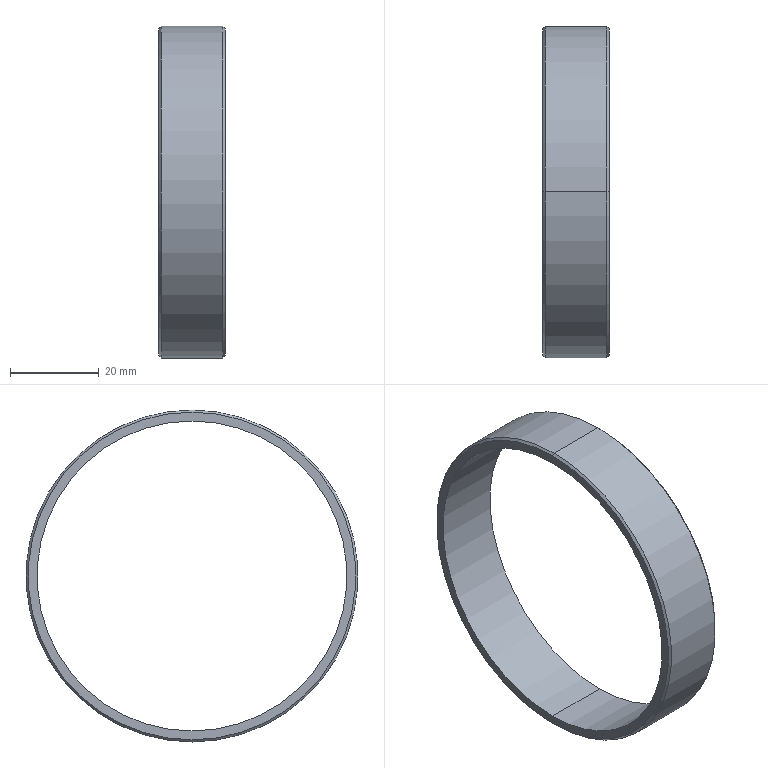Part | SolidWorks | features Chamfer 1, Extrusion 1 | 1 solid | 10 faces | box 15 x 75 x 75 mm | volume 8483 mm3 | cone 4 | cylinder 4 | plane 2 | commonest cylinder face diameters 70 x2 75 x2
STEP:
#1=CARTESIAN_POINT('',(0.,0.,-37.));
#2=VERTEX_POINT('',#1);
#3=CARTESIAN_POINT('',(0.,0.,37.));
#4=VERTEX_POINT('',#3);
#5=CARTESIAN_POINT('',(0.,0.,0.));
#6=DIRECTION('',(1.,0.,0.));
#7=DIRECTION('',(0.,0.,-1.));
#8=AXIS2_PLACEMENT_3D('',#5,#6,#7);
#9=CIRCLE('',#8,37.);
#10=EDGE_CURVE('',#2,#4,#9,.T.);
#11=ORIENTED_EDGE('',*,*,#10,.F.);
#12=CARTESIAN_POINT('',(-0.5,0.,-37.5));
#13=VERTEX_POINT('',#12);
#14=CARTESIAN_POINT('',(0.,0.,-37.));
#15=DIRECTION('',(-0.7071,0.,-0.7071));
#16=VECTOR('',#15,1000.);
#17=LINE('',#14,#16);
#18=EDGE_CURVE('',#2,#13,#17,.T.);
#19=ORIENTED_EDGE('',*,*,#18,.T.);
#20=CARTESIAN_POINT('',(-0.5,0.,37.5));
#21=VERTEX_POINT('',#20);
#22=CARTESIAN_POINT('',(-0.5,0.,0.));
#23=DIRECTION('',(-1.,0.,0.));
#24=DIRECTION('',(0.,0.,-1.));
#25=AXIS2_PLACEMENT_3D('',#22,#23,#24);
#26=CIRCLE('',#25,37.5);
#27=EDGE_CURVE('',#21,#13,#26,.T.);
#28=ORIENTED_EDGE('',*,*,#27,.F.);
#29=CARTESIAN_POINT('',(0.,0.,37.));
#30=DIRECTION('',(-0.7071,0.,0.7071));
#31=VECTOR('',#30,1000.);
#32=LINE('',#29,#31);
#33=EDGE_CURVE('',#4,#21,#32,.T.);
#34=ORIENTED_EDGE('',*,*,#33,.F.);
#35=EDGE_LOOP('',(#11,#19,#28,#34));
#36=FACE_OUTER_BOUND('',#35,.T.);
#37=CARTESIAN_POINT('',(0.,0.,0.));
#38=DIRECTION('',(-1.,0.,0.));
#39=DIRECTION('',(0.,0.,1.));
#40=AXIS2_PLACEMENT_3D('',#37,#38,#39);
#41=CONICAL_SURFACE('',#40,37.,0.7854);
#42=ADVANCED_FACE('',(#36),#41,.T.);
#43=CARTESIAN_POINT('',(-15.,0.,37.));
#44=VERTEX_POINT('',#43);
#45=CARTESIAN_POINT('',(-15.,0.,-37.));
#46=VERTEX_POINT('',#45);
#47=CARTESIAN_POINT('',(-15.,0.,0.));
#48=DIRECTION('',(-1.,0.,0.));
#49=DIRECTION('',(0.,0.,-1.));
#50=AXIS2_PLACEMENT_3D('',#47,#48,#49);
#51=CIRCLE('',#50,37.);
#52=EDGE_CURVE('',#44,#46,#51,.T.);
#53=ORIENTED_EDGE('',*,*,#52,.F.);
#54=CARTESIAN_POINT('',(-14.5,0.,37.5));
#55=VERTEX_POINT('',#54);
#56=CARTESIAN_POINT('',(-14.5,0.,37.5));
#57=DIRECTION('',(0.7071,0.,0.7071));
#58=VECTOR('',#57,1000.);
#59=LINE('',#56,#58);
#60=EDGE_CURVE('',#44,#55,#59,.T.);
#61=ORIENTED_EDGE('',*,*,#60,.T.);
#62=CARTESIAN_POINT('',(-14.5,0.,-37.5));
#63=VERTEX_POINT('',#62);
#64=CARTESIAN_POINT('',(-14.5,0.,0.));
#65=DIRECTION('',(1.,0.,0.));
#66=DIRECTION('',(0.,0.,-1.));
#67=AXIS2_PLACEMENT_3D('',#64,#65,#66);
#68=CIRCLE('',#67,37.5);
#69=EDGE_CURVE('',#63,#55,#68,.T.);
#70=ORIENTED_EDGE('',*,*,#69,.F.);
#71=CARTESIAN_POINT('',(-14.5,0.,-37.5));
#72=DIRECTION('',(0.7071,0.,-0.7071));
#73=VECTOR('',#72,1000.);
#74=LINE('',#71,#73);
#75=EDGE_CURVE('',#46,#63,#74,.T.);
#76=ORIENTED_EDGE('',*,*,#75,.F.);
#77=EDGE_LOOP('',(#53,#61,#70,#76));
#78=FACE_OUTER_BOUND('',#77,.T.);
#79=CARTESIAN_POINT('',(-14.5,0.,0.));
#80=DIRECTION('',(1.,0.,0.));
#81=DIRECTION('',(0.,0.,-1.));
#82=AXIS2_PLACEMENT_3D('',#79,#80,#81);
#83=CONICAL_SURFACE('',#82,37.5,0.7854);
#84=ADVANCED_FACE('',(#78),#83,.T.);
#85=CARTESIAN_POINT('',(-15.,0.,35.));
#86=VERTEX_POINT('',#85);
#87=CARTESIAN_POINT('',(-15.,0.,-35.));
#88=VERTEX_POINT('',#87);
#89=CARTESIAN_POINT('',(-15.,0.,0.));
#90=DIRECTION('',(1.,0.,0.));
#91=DIRECTION('',(0.,0.,-1.));
#92=AXIS2_PLACEMENT_3D('',#89,#90,#91);
#93=CIRCLE('',#92,35.);
#94=EDGE_CURVE('',#86,#88,#93,.T.);
#95=ORIENTED_EDGE('',*,*,#94,.F.);
#96=CARTESIAN_POINT('',(0.,0.,35.));
#97=VERTEX_POINT('',#96);
#98=CARTESIAN_POINT('',(-15.,0.,35.));
#99=DIRECTION('',(1.,0.,0.));
#100=VECTOR('',#99,1000.);
#101=LINE('',#98,#100);
#102=EDGE_CURVE('',#86,#97,#101,.T.);
#103=ORIENTED_EDGE('',*,*,#102,.T.);
#104=CARTESIAN_POINT('',(0.,0.,-35.));
#105=VERTEX_POINT('',#104);
#106=CARTESIAN_POINT('',(0.,0.,0.));
#107=DIRECTION('',(1.,0.,0.));
#108=DIRECTION('',(0.,0.,-1.));
#109=AXIS2_PLACEMENT_3D('',#106,#107,#108);
#110=CIRCLE('',#109,35.);
#111=EDGE_CURVE('',#97,#105,#110,.T.);
#112=ORIENTED_EDGE('',*,*,#111,.T.);
#113=CARTESIAN_POINT('',(-15.,0.,-35.));
#114=DIRECTION('',(1.,0.,0.));
#115=VECTOR('',#114,1000.);
#116=LINE('',#113,#115);
#117=EDGE_CURVE('',#88,#105,#116,.T.);
#118=ORIENTED_EDGE('',*,*,#117,.F.);
#119=EDGE_LOOP('',(#95,#103,#112,#118));
#120=FACE_OUTER_BOUND('',#119,.T.);
#121=CARTESIAN_POINT('',(-15.,0.,0.));
#122=DIRECTION('',(1.,0.,0.));
#123=DIRECTION('',(0.,0.,-1.));
#124=AXIS2_PLACEMENT_3D('',#121,#122,#123);
#125=CYLINDRICAL_SURFACE('',#124,35.);
#126=ADVANCED_FACE('',(#120),#125,.F.);
#127=ORIENTED_EDGE('',*,*,#69,.T.);
#128=CARTESIAN_POINT('',(-15.,0.,37.5));
#129=DIRECTION('',(1.,0.,0.));
#130=VECTOR('',#129,1000.);
#131=LINE('',#128,#130);
#132=EDGE_CURVE('',#55,#21,#131,.T.);
#133=ORIENTED_EDGE('',*,*,#132,.T.);
#134=ORIENTED_EDGE('',*,*,#27,.T.);
#135=CARTESIAN_POINT('',(-15.,0.,-37.5));
#136=DIRECTION('',(1.,0.,0.));
#137=VECTOR('',#136,1000.);
#138=LINE('',#135,#137);
#139=EDGE_CURVE('',#63,#13,#138,.T.);
#140=ORIENTED_EDGE('',*,*,#139,.F.);
#141=EDGE_LOOP('',(#127,#133,#134,#140));
#142=FACE_OUTER_BOUND('',#141,.T.);
#143=CARTESIAN_POINT('',(-15.,0.,0.));
#144=DIRECTION('',(1.,0.,0.));
#145=DIRECTION('',(0.,0.,-1.));
#146=AXIS2_PLACEMENT_3D('',#143,#144,#145);
#147=CYLINDRICAL_SURFACE('',#146,37.5);
#148=ADVANCED_FACE('',(#142),#147,.T.);
#149=ORIENTED_EDGE('',*,*,#132,.F.);
#150=CARTESIAN_POINT('',(-14.5,0.,0.));
#151=DIRECTION('',(1.,0.,0.));
#152=DIRECTION('',(0.,0.,-1.));
#153=AXIS2_PLACEMENT_3D('',#150,#151,#152);
#154=CIRCLE('',#153,37.5);
#155=EDGE_CURVE('',#55,#63,#154,.T.);
#156=ORIENTED_EDGE('',*,*,#155,.T.);
#157=ORIENTED_EDGE('',*,*,#139,.T.);
#158=CARTESIAN_POINT('',(-0.5,0.,0.));
#159=DIRECTION('',(-1.,0.,0.));
#160=DIRECTION('',(0.,0.,-1.));
#161=AXIS2_PLACEMENT_3D('',#158,#159,#160);
#162=CIRCLE('',#161,37.5);
#163=EDGE_CURVE('',#13,#21,#162,.T.);
#164=ORIENTED_EDGE('',*,*,#163,.T.);
#165=EDGE_LOOP('',(#149,#156,#157,#164));
#166=FACE_OUTER_BOUND('',#165,.T.);
#167=CARTESIAN_POINT('',(-15.,0.,0.));
#168=DIRECTION('',(1.,0.,0.));
#169=DIRECTION('',(0.,0.,-1.));
#170=AXIS2_PLACEMENT_3D('',#167,#168,#169);
#171=CYLINDRICAL_SURFACE('',#170,37.5);
#172=ADVANCED_FACE('',(#166),#171,.T.);
#173=CARTESIAN_POINT('',(-15.,0.,0.));
#174=DIRECTION('',(-1.,0.,0.));
#175=DIRECTION('',(0.,0.,-1.));
#176=AXIS2_PLACEMENT_3D('',#173,#174,#175);
#177=CIRCLE('',#176,37.);
#178=EDGE_CURVE('',#46,#44,#177,.T.);
#179=ORIENTED_EDGE('',*,*,#178,.T.);
#180=ORIENTED_EDGE('',*,*,#52,.T.);
#181=EDGE_LOOP('',(#179,#180));
#182=FACE_OUTER_BOUND('',#181,.T.);
#183=CARTESIAN_POINT('',(-15.,0.,0.));
#184=DIRECTION('',(1.,0.,0.));
#185=DIRECTION('',(0.,0.,-1.));
#186=AXIS2_PLACEMENT_3D('',#183,#184,#185);
#187=CIRCLE('',#186,35.);
#188=EDGE_CURVE('',#88,#86,#187,.T.);
#189=ORIENTED_EDGE('',*,*,#188,.T.);
#190=ORIENTED_EDGE('',*,*,#94,.T.);
#191=EDGE_LOOP('',(#189,#190));
#192=FACE_BOUND('',#191,.T.);
#193=CARTESIAN_POINT('',(-15.,0.,0.));
#194=DIRECTION('',(1.,0.,0.));
#195=DIRECTION('',(0.,0.,-1.));
#196=AXIS2_PLACEMENT_3D('',#193,#194,#195);
#197=PLANE('',#196);
#198=ADVANCED_FACE('',(#182,#192),#197,.F.);
#199=CARTESIAN_POINT('',(0.,0.,0.));
#200=DIRECTION('',(1.,0.,0.));
#201=DIRECTION('',(0.,0.,-1.));
#202=AXIS2_PLACEMENT_3D('',#199,#200,#201);
#203=CIRCLE('',#202,37.);
#204=EDGE_CURVE('',#4,#2,#203,.T.);
#205=ORIENTED_EDGE('',*,*,#204,.T.);
#206=ORIENTED_EDGE('',*,*,#10,.T.);
#207=EDGE_LOOP('',(#205,#206));
#208=FACE_OUTER_BOUND('',#207,.T.);
#209=CARTESIAN_POINT('',(0.,0.,0.));
#210=DIRECTION('',(1.,0.,0.));
#211=DIRECTION('',(0.,0.,-1.));
#212=AXIS2_PLACEMENT_3D('',#209,#210,#211);
#213=CIRCLE('',#212,35.);
#214=EDGE_CURVE('',#105,#97,#213,.T.);
#215=ORIENTED_EDGE('',*,*,#214,.F.);
#216=ORIENTED_EDGE('',*,*,#111,.F.);
#217=EDGE_LOOP('',(#215,#216));
#218=FACE_BOUND('',#217,.T.);
#219=CARTESIAN_POINT('',(0.,0.,0.));
#220=DIRECTION('',(1.,0.,0.));
#221=DIRECTION('',(0.,0.,-1.));
#222=AXIS2_PLACEMENT_3D('',#219,#220,#221);
#223=PLANE('',#222);
#224=ADVANCED_FACE('',(#208,#218),#223,.T.);
#225=ORIENTED_EDGE('',*,*,#102,.F.);
#226=ORIENTED_EDGE('',*,*,#188,.F.);
#227=ORIENTED_EDGE('',*,*,#117,.T.);
#228=ORIENTED_EDGE('',*,*,#214,.T.);
#229=EDGE_LOOP('',(#225,#226,#227,#228));
#230=FACE_OUTER_BOUND('',#229,.T.);
#231=CARTESIAN_POINT('',(-15.,0.,0.));
#232=DIRECTION('',(1.,0.,0.));
#233=DIRECTION('',(0.,0.,-1.));
#234=AXIS2_PLACEMENT_3D('',#231,#232,#233);
#235=CYLINDRICAL_SURFACE('',#234,35.);
#236=ADVANCED_FACE('',(#230),#235,.F.);
#237=ORIENTED_EDGE('',*,*,#60,.F.);
#238=ORIENTED_EDGE('',*,*,#178,.F.);
#239=ORIENTED_EDGE('',*,*,#75,.T.);
#240=ORIENTED_EDGE('',*,*,#155,.F.);
#241=EDGE_LOOP('',(#237,#238,#239,#240));
#242=FACE_OUTER_BOUND('',#241,.T.);
#243=CARTESIAN_POINT('',(-14.5,0.,0.));
#244=DIRECTION('',(1.,0.,0.));
#245=DIRECTION('',(0.,0.,-1.));
#246=AXIS2_PLACEMENT_3D('',#243,#244,#245);
#247=CONICAL_SURFACE('',#246,37.5,0.7854);
#248=ADVANCED_FACE('',(#242),#247,.T.);
#249=ORIENTED_EDGE('',*,*,#18,.F.);
#250=ORIENTED_EDGE('',*,*,#204,.F.);
#251=ORIENTED_EDGE('',*,*,#33,.T.);
#252=ORIENTED_EDGE('',*,*,#163,.F.);
#253=EDGE_LOOP('',(#249,#250,#251,#252));
#254=FACE_OUTER_BOUND('',#253,.T.);
#255=CARTESIAN_POINT('',(0.,0.,0.));
#256=DIRECTION('',(-1.,0.,0.));
#257=DIRECTION('',(0.,0.,1.));
#258=AXIS2_PLACEMENT_3D('',#255,#256,#257);
#259=CONICAL_SURFACE('',#258,37.,0.7854);
#260=ADVANCED_FACE('',(#254),#259,.T.);
#261=CLOSED_SHELL('',(#42,#84,#126,#148,#172,#198,#224,#236,#248,#260));
#262=MANIFOLD_SOLID_BREP('',#261);
#263=CARTESIAN_POINT('',(0.,0.,0.));
#264=DIRECTION('',(0.,0.,1.));
#265=DIRECTION('',(1.,0.,0.));
#266=AXIS2_PLACEMENT_3D('',#263,#264,#265);
#267=(LENGTH_UNIT()NAMED_UNIT(*)SI_UNIT(.MILLI.,.METRE.));
#268=UNCERTAINTY_MEASURE_WITH_UNIT(LENGTH_MEASURE(0.00001),#267,'','');
#269=(NAMED_UNIT(*)PLANE_ANGLE_UNIT()SI_UNIT($,.RADIAN.));
#270=(NAMED_UNIT(*)SI_UNIT($,.STERADIAN.)SOLID_ANGLE_UNIT());
#271=(GEOMETRIC_REPRESENTATION_CONTEXT(3)GLOBAL_UNCERTAINTY_ASSIGNED_CONTEXT((#268))GLOBAL_UNIT_ASSIGNED_CONTEXT((#267,#269,#270))REPRESENTATION_CONTEXT('',''));
#272=ADVANCED_BREP_SHAPE_REPRESENTATION('',(#262,#266),#271);